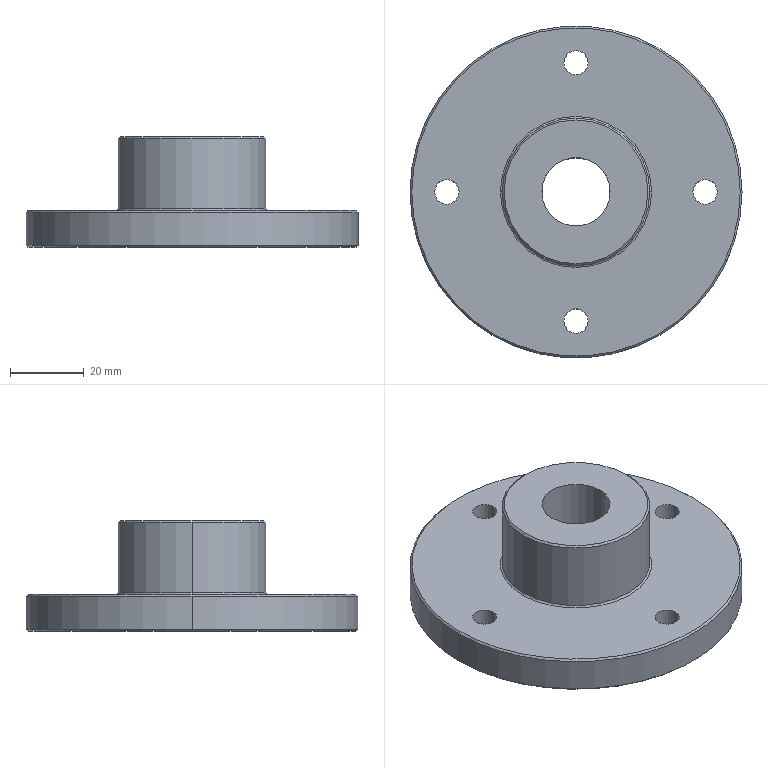Part | STEP file | 44-02-24 Press Cylinder Connector | 1 solid | 25 faces | box 90 x 90 x 30 mm | volume 79238 mm3 | cylinder 14 | cone 6 | plane 3 | torus 2 | commonest cylinder face diameters 6.6 x8 18.5 x2 40 x2 90 x2